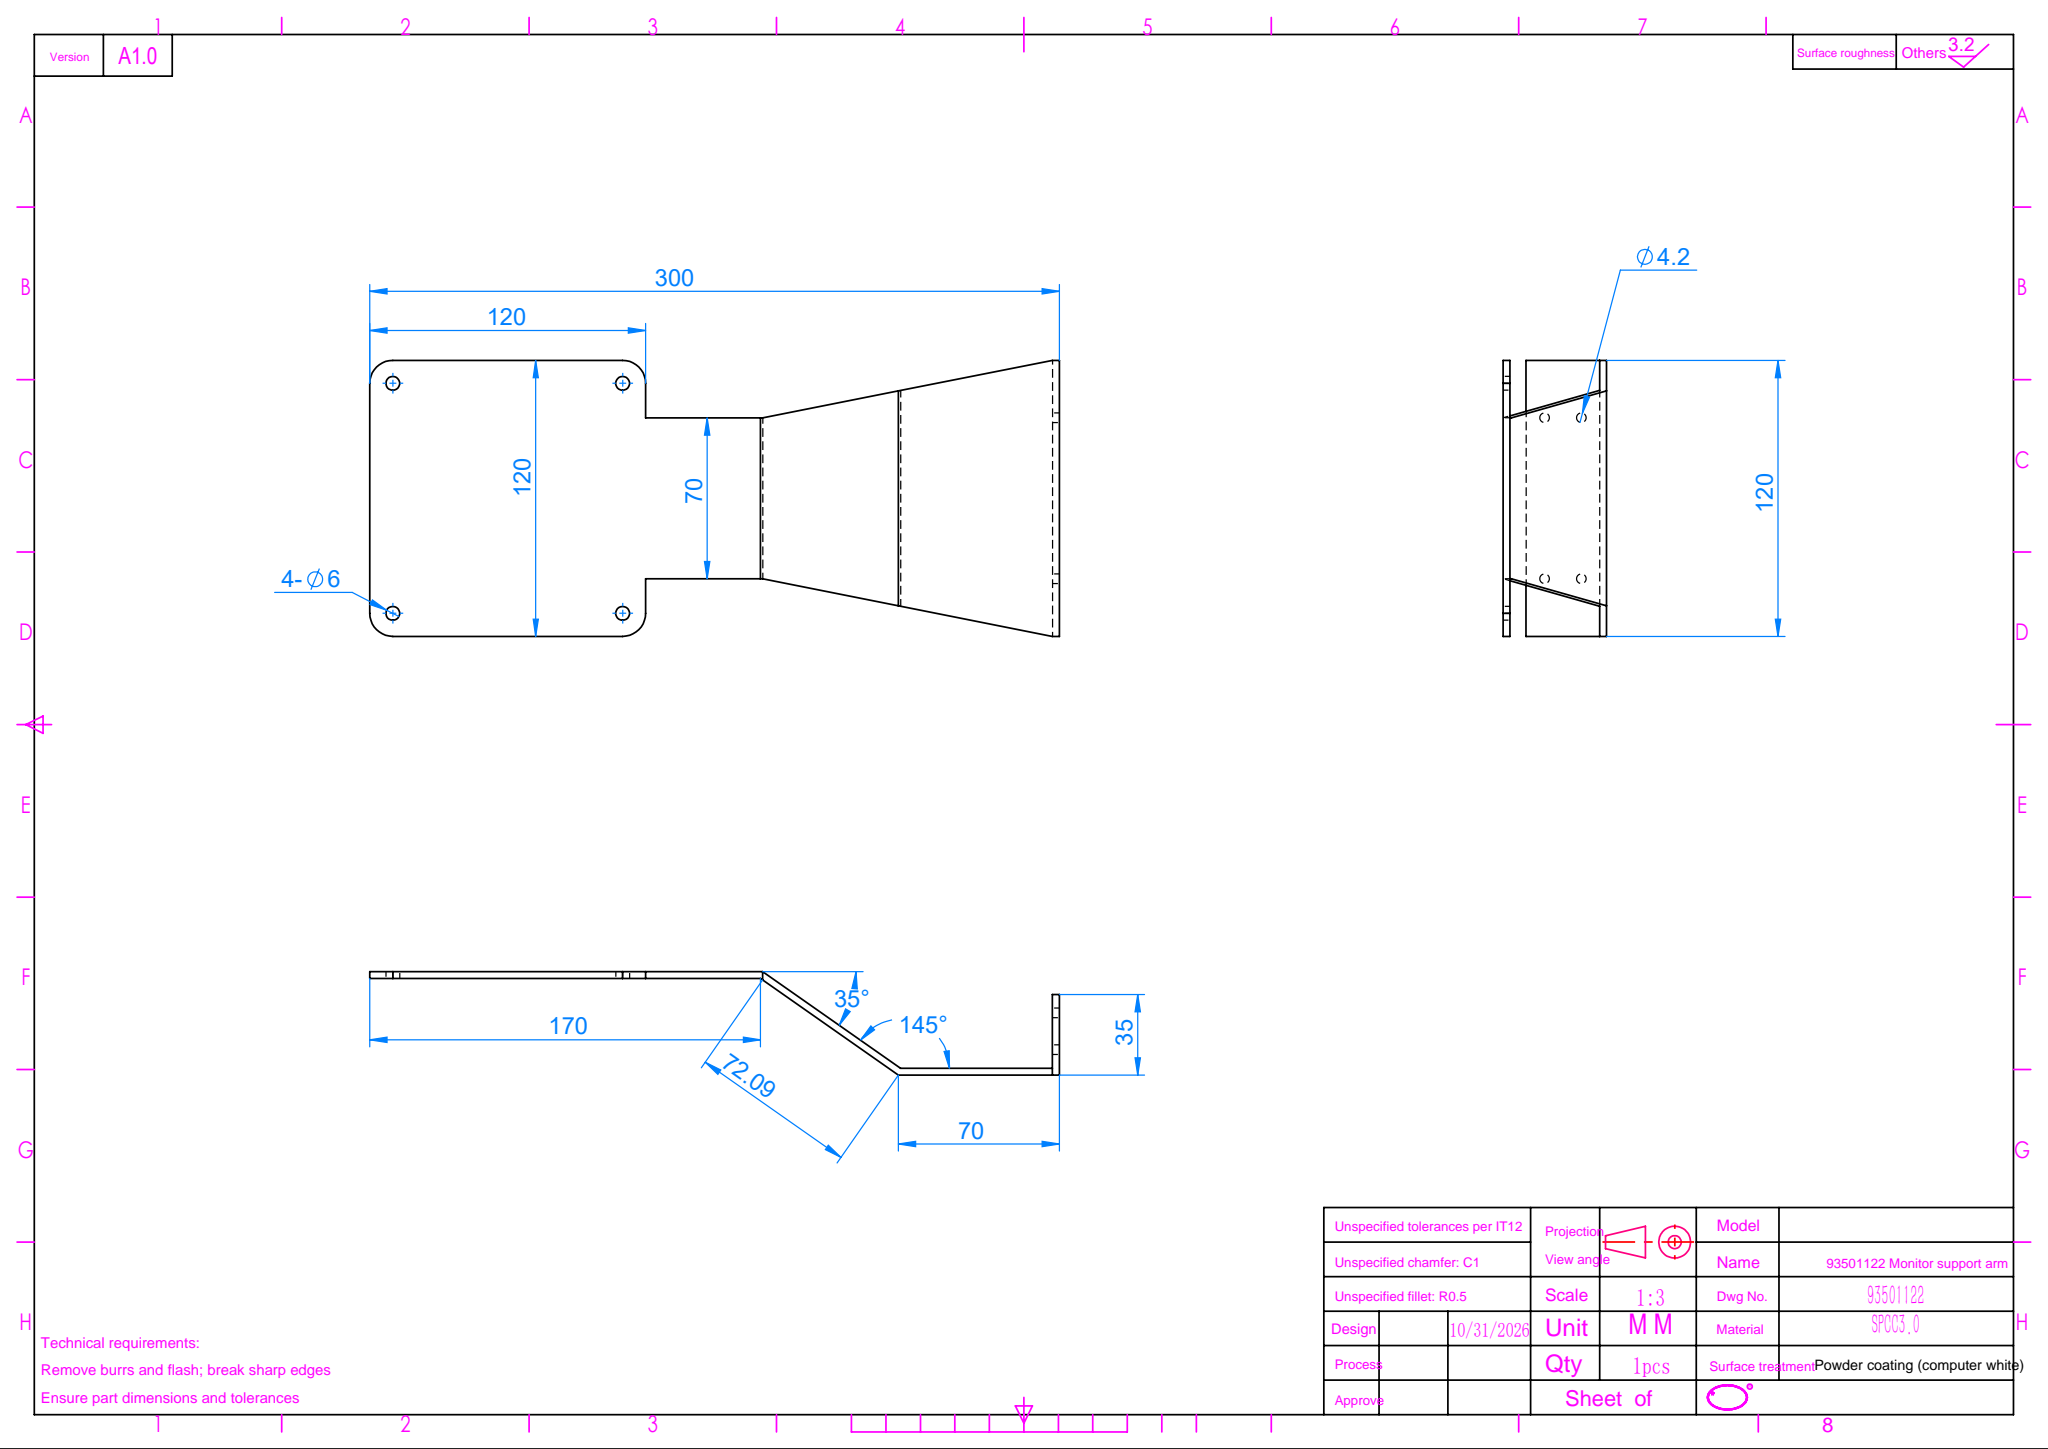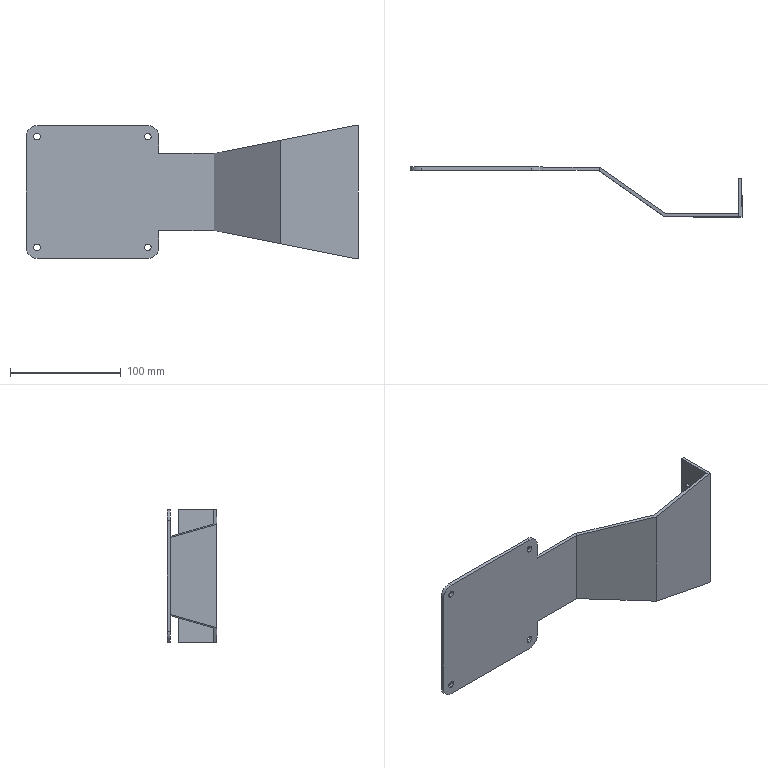Part | SolidWorks | features ICE 3, ExtruThin 1, Fillet 1 | 1 solid | 40 faces | box 300 x 45 x 120 mm | volume 104906 mm3 | cylinder 20 | plane 20 | commonest cylinder face diameters 4.2 x8 6 x8 20 x4